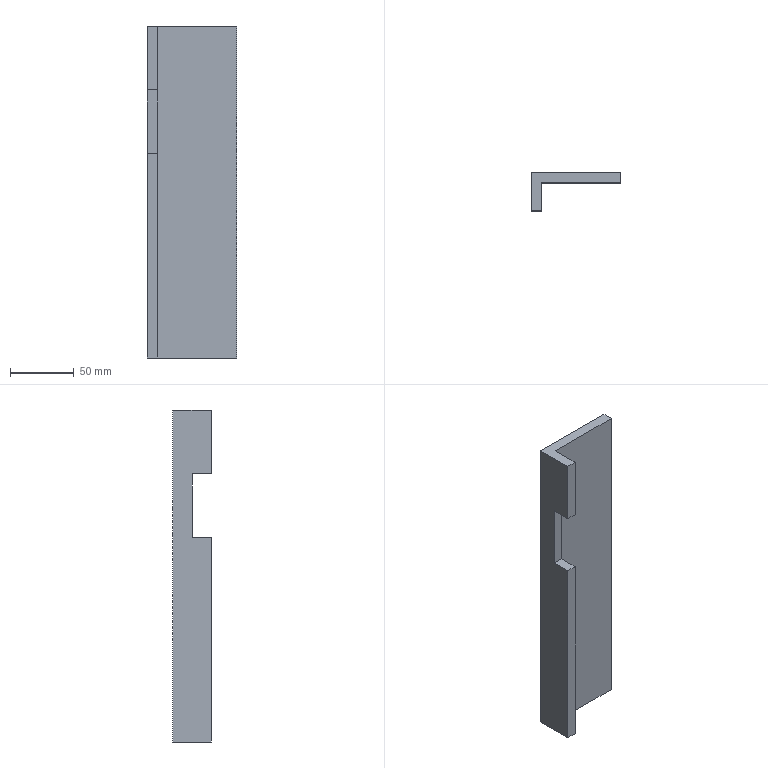Part | SolidWorks | features Cut 1, Extrusion 1 | 1 solid | 12 faces | box 70 x 30 x 260 mm | volume 185360 mm3 | plane 12
STEP:
#1=CARTESIAN_POINT('',(0.,-30.,260.));
#2=VERTEX_POINT('',#1);
#3=CARTESIAN_POINT('',(0.,-30.,210.));
#4=VERTEX_POINT('',#3);
#5=CARTESIAN_POINT('',(0.,-30.,260.));
#6=DIRECTION('',(0.,0.,-1.));
#7=VECTOR('',#6,1000.);
#8=LINE('',#5,#7);
#9=EDGE_CURVE('',#2,#4,#8,.T.);
#10=ORIENTED_EDGE('',*,*,#9,.T.);
#11=CARTESIAN_POINT('',(8.,-30.,210.));
#12=VERTEX_POINT('',#11);
#13=CARTESIAN_POINT('',(10.,-30.,210.));
#14=DIRECTION('',(-1.,0.,0.));
#15=VECTOR('',#14,1000.);
#16=LINE('',#13,#15);
#17=EDGE_CURVE('',#12,#4,#16,.T.);
#18=ORIENTED_EDGE('',*,*,#17,.F.);
#19=CARTESIAN_POINT('',(8.,-30.,260.));
#20=VERTEX_POINT('',#19);
#21=CARTESIAN_POINT('',(8.,-30.,260.));
#22=DIRECTION('',(0.,0.,-1.));
#23=VECTOR('',#22,1000.);
#24=LINE('',#21,#23);
#25=EDGE_CURVE('',#20,#12,#24,.T.);
#26=ORIENTED_EDGE('',*,*,#25,.F.);
#27=CARTESIAN_POINT('',(0.,-30.,260.));
#28=DIRECTION('',(1.,0.,0.));
#29=VECTOR('',#28,1000.);
#30=LINE('',#27,#29);
#31=EDGE_CURVE('',#2,#20,#30,.T.);
#32=ORIENTED_EDGE('',*,*,#31,.F.);
#33=EDGE_LOOP('',(#10,#18,#26,#32));
#34=FACE_OUTER_BOUND('',#33,.T.);
#35=CARTESIAN_POINT('',(0.,-30.,260.));
#36=DIRECTION('',(0.,1.,0.));
#37=DIRECTION('',(0.,0.,1.));
#38=AXIS2_PLACEMENT_3D('',#35,#36,#37);
#39=PLANE('',#38);
#40=ADVANCED_FACE('',(#34),#39,.F.);
#41=CARTESIAN_POINT('',(0.,-15.,210.));
#42=VERTEX_POINT('',#41);
#43=CARTESIAN_POINT('',(0.,-15.,160.));
#44=VERTEX_POINT('',#43);
#45=CARTESIAN_POINT('',(0.,-15.,0.));
#46=DIRECTION('',(0.,0.,-1.));
#47=VECTOR('',#46,1000.);
#48=LINE('',#45,#47);
#49=EDGE_CURVE('',#42,#44,#48,.T.);
#50=ORIENTED_EDGE('',*,*,#49,.F.);
#51=CARTESIAN_POINT('',(0.,0.,210.));
#52=DIRECTION('',(0.,1.,0.));
#53=VECTOR('',#52,1000.);
#54=LINE('',#51,#53);
#55=EDGE_CURVE('',#4,#42,#54,.T.);
#56=ORIENTED_EDGE('',*,*,#55,.F.);
#57=ORIENTED_EDGE('',*,*,#9,.F.);
#58=CARTESIAN_POINT('',(0.,0.,260.));
#59=VERTEX_POINT('',#58);
#60=CARTESIAN_POINT('',(0.,0.,260.));
#61=DIRECTION('',(0.,-1.,0.));
#62=VECTOR('',#61,1000.);
#63=LINE('',#60,#62);
#64=EDGE_CURVE('',#59,#2,#63,.T.);
#65=ORIENTED_EDGE('',*,*,#64,.F.);
#66=CARTESIAN_POINT('',(0.,0.,0.));
#67=VERTEX_POINT('',#66);
#68=CARTESIAN_POINT('',(0.,0.,260.));
#69=DIRECTION('',(0.,0.,-1.));
#70=VECTOR('',#69,1000.);
#71=LINE('',#68,#70);
#72=EDGE_CURVE('',#59,#67,#71,.T.);
#73=ORIENTED_EDGE('',*,*,#72,.T.);
#74=CARTESIAN_POINT('',(0.,-30.,0.));
#75=VERTEX_POINT('',#74);
#76=CARTESIAN_POINT('',(0.,0.,0.));
#77=DIRECTION('',(0.,-1.,0.));
#78=VECTOR('',#77,1000.);
#79=LINE('',#76,#78);
#80=EDGE_CURVE('',#67,#75,#79,.T.);
#81=ORIENTED_EDGE('',*,*,#80,.T.);
#82=CARTESIAN_POINT('',(0.,-30.,160.));
#83=VERTEX_POINT('',#82);
#84=CARTESIAN_POINT('',(0.,-30.,260.));
#85=DIRECTION('',(0.,0.,-1.));
#86=VECTOR('',#85,1000.);
#87=LINE('',#84,#86);
#88=EDGE_CURVE('',#83,#75,#87,.T.);
#89=ORIENTED_EDGE('',*,*,#88,.F.);
#90=CARTESIAN_POINT('',(0.,0.,160.));
#91=DIRECTION('',(0.,-1.,0.));
#92=VECTOR('',#91,1000.);
#93=LINE('',#90,#92);
#94=EDGE_CURVE('',#44,#83,#93,.T.);
#95=ORIENTED_EDGE('',*,*,#94,.F.);
#96=EDGE_LOOP('',(#50,#56,#57,#65,#73,#81,#89,#95));
#97=FACE_OUTER_BOUND('',#96,.T.);
#98=CARTESIAN_POINT('',(0.,0.,260.));
#99=DIRECTION('',(1.,0.,0.));
#100=DIRECTION('',(0.,1.,0.));
#101=AXIS2_PLACEMENT_3D('',#98,#99,#100);
#102=PLANE('',#101);
#103=ADVANCED_FACE('',(#97),#102,.F.);
#104=CARTESIAN_POINT('',(8.,-30.,160.));
#105=VERTEX_POINT('',#104);
#106=CARTESIAN_POINT('',(8.,-30.,0.));
#107=VERTEX_POINT('',#106);
#108=CARTESIAN_POINT('',(8.,-30.,260.));
#109=DIRECTION('',(0.,0.,-1.));
#110=VECTOR('',#109,1000.);
#111=LINE('',#108,#110);
#112=EDGE_CURVE('',#105,#107,#111,.T.);
#113=ORIENTED_EDGE('',*,*,#112,.F.);
#114=CARTESIAN_POINT('',(10.,-30.,160.));
#115=DIRECTION('',(-1.,0.,0.));
#116=VECTOR('',#115,1000.);
#117=LINE('',#114,#116);
#118=EDGE_CURVE('',#105,#83,#117,.T.);
#119=ORIENTED_EDGE('',*,*,#118,.T.);
#120=ORIENTED_EDGE('',*,*,#88,.T.);
#121=CARTESIAN_POINT('',(0.,-30.,0.));
#122=DIRECTION('',(1.,0.,0.));
#123=VECTOR('',#122,1000.);
#124=LINE('',#121,#123);
#125=EDGE_CURVE('',#75,#107,#124,.T.);
#126=ORIENTED_EDGE('',*,*,#125,.T.);
#127=EDGE_LOOP('',(#113,#119,#120,#126));
#128=FACE_OUTER_BOUND('',#127,.T.);
#129=CARTESIAN_POINT('',(0.,-30.,260.));
#130=DIRECTION('',(0.,1.,0.));
#131=DIRECTION('',(0.,0.,1.));
#132=AXIS2_PLACEMENT_3D('',#129,#130,#131);
#133=PLANE('',#132);
#134=ADVANCED_FACE('',(#128),#133,.F.);
#135=ORIENTED_EDGE('',*,*,#25,.T.);
#136=CARTESIAN_POINT('',(8.,-15.,210.));
#137=VERTEX_POINT('',#136);
#138=CARTESIAN_POINT('',(8.,-8.,210.));
#139=DIRECTION('',(0.,1.,0.));
#140=VECTOR('',#139,1000.);
#141=LINE('',#138,#140);
#142=EDGE_CURVE('',#12,#137,#141,.T.);
#143=ORIENTED_EDGE('',*,*,#142,.T.);
#144=CARTESIAN_POINT('',(8.,-15.,160.));
#145=VERTEX_POINT('',#144);
#146=CARTESIAN_POINT('',(8.,-15.,260.));
#147=DIRECTION('',(0.,0.,-1.));
#148=VECTOR('',#147,1000.);
#149=LINE('',#146,#148);
#150=EDGE_CURVE('',#137,#145,#149,.T.);
#151=ORIENTED_EDGE('',*,*,#150,.T.);
#152=CARTESIAN_POINT('',(8.,-8.,160.));
#153=DIRECTION('',(0.,-1.,0.));
#154=VECTOR('',#153,1000.);
#155=LINE('',#152,#154);
#156=EDGE_CURVE('',#145,#105,#155,.T.);
#157=ORIENTED_EDGE('',*,*,#156,.T.);
#158=ORIENTED_EDGE('',*,*,#112,.T.);
#159=CARTESIAN_POINT('',(8.,-8.,0.));
#160=VERTEX_POINT('',#159);
#161=CARTESIAN_POINT('',(8.,-8.,0.));
#162=DIRECTION('',(0.,1.,0.));
#163=VECTOR('',#162,1000.);
#164=LINE('',#161,#163);
#165=EDGE_CURVE('',#107,#160,#164,.T.);
#166=ORIENTED_EDGE('',*,*,#165,.T.);
#167=CARTESIAN_POINT('',(8.,-8.,260.));
#168=VERTEX_POINT('',#167);
#169=CARTESIAN_POINT('',(8.,-8.,260.));
#170=DIRECTION('',(0.,0.,-1.));
#171=VECTOR('',#170,1000.);
#172=LINE('',#169,#171);
#173=EDGE_CURVE('',#168,#160,#172,.T.);
#174=ORIENTED_EDGE('',*,*,#173,.F.);
#175=CARTESIAN_POINT('',(8.,-8.,260.));
#176=DIRECTION('',(0.,1.,0.));
#177=VECTOR('',#176,1000.);
#178=LINE('',#175,#177);
#179=EDGE_CURVE('',#20,#168,#178,.T.);
#180=ORIENTED_EDGE('',*,*,#179,.F.);
#181=EDGE_LOOP('',(#135,#143,#151,#157,#158,#166,#174,#180));
#182=FACE_OUTER_BOUND('',#181,.T.);
#183=CARTESIAN_POINT('',(8.,-8.,260.));
#184=DIRECTION('',(-1.,0.,0.));
#185=DIRECTION('',(0.,0.,1.));
#186=AXIS2_PLACEMENT_3D('',#183,#184,#185);
#187=PLANE('',#186);
#188=ADVANCED_FACE('',(#182),#187,.F.);
#189=CARTESIAN_POINT('',(70.,-8.,0.));
#190=VERTEX_POINT('',#189);
#191=CARTESIAN_POINT('',(8.,-8.,0.));
#192=DIRECTION('',(1.,0.,0.));
#193=VECTOR('',#192,1000.);
#194=LINE('',#191,#193);
#195=EDGE_CURVE('',#160,#190,#194,.T.);
#196=ORIENTED_EDGE('',*,*,#195,.T.);
#197=CARTESIAN_POINT('',(70.,-8.,260.));
#198=VERTEX_POINT('',#197);
#199=CARTESIAN_POINT('',(70.,-8.,260.));
#200=DIRECTION('',(0.,0.,-1.));
#201=VECTOR('',#200,1000.);
#202=LINE('',#199,#201);
#203=EDGE_CURVE('',#198,#190,#202,.T.);
#204=ORIENTED_EDGE('',*,*,#203,.F.);
#205=CARTESIAN_POINT('',(8.,-8.,260.));
#206=DIRECTION('',(1.,0.,0.));
#207=VECTOR('',#206,1000.);
#208=LINE('',#205,#207);
#209=EDGE_CURVE('',#168,#198,#208,.T.);
#210=ORIENTED_EDGE('',*,*,#209,.F.);
#211=ORIENTED_EDGE('',*,*,#173,.T.);
#212=EDGE_LOOP('',(#196,#204,#210,#211));
#213=FACE_OUTER_BOUND('',#212,.T.);
#214=CARTESIAN_POINT('',(8.,-8.,260.));
#215=DIRECTION('',(0.,1.,0.));
#216=DIRECTION('',(0.,0.,1.));
#217=AXIS2_PLACEMENT_3D('',#214,#215,#216);
#218=PLANE('',#217);
#219=ADVANCED_FACE('',(#213),#218,.F.);
#220=CARTESIAN_POINT('',(70.,0.,0.));
#221=VERTEX_POINT('',#220);
#222=CARTESIAN_POINT('',(70.,-8.,0.));
#223=DIRECTION('',(0.,1.,0.));
#224=VECTOR('',#223,1000.);
#225=LINE('',#222,#224);
#226=EDGE_CURVE('',#190,#221,#225,.T.);
#227=ORIENTED_EDGE('',*,*,#226,.T.);
#228=CARTESIAN_POINT('',(70.,0.,260.));
#229=VERTEX_POINT('',#228);
#230=CARTESIAN_POINT('',(70.,0.,260.));
#231=DIRECTION('',(0.,0.,-1.));
#232=VECTOR('',#231,1000.);
#233=LINE('',#230,#232);
#234=EDGE_CURVE('',#229,#221,#233,.T.);
#235=ORIENTED_EDGE('',*,*,#234,.F.);
#236=CARTESIAN_POINT('',(70.,-8.,260.));
#237=DIRECTION('',(0.,1.,0.));
#238=VECTOR('',#237,1000.);
#239=LINE('',#236,#238);
#240=EDGE_CURVE('',#198,#229,#239,.T.);
#241=ORIENTED_EDGE('',*,*,#240,.F.);
#242=ORIENTED_EDGE('',*,*,#203,.T.);
#243=EDGE_LOOP('',(#227,#235,#241,#242));
#244=FACE_OUTER_BOUND('',#243,.T.);
#245=CARTESIAN_POINT('',(70.,-8.,260.));
#246=DIRECTION('',(-1.,0.,0.));
#247=DIRECTION('',(0.,0.,1.));
#248=AXIS2_PLACEMENT_3D('',#245,#246,#247);
#249=PLANE('',#248);
#250=ADVANCED_FACE('',(#244),#249,.F.);
#251=CARTESIAN_POINT('',(0.,0.,0.));
#252=DIRECTION('',(-1.,0.,0.));
#253=VECTOR('',#252,1000.);
#254=LINE('',#251,#253);
#255=EDGE_CURVE('',#221,#67,#254,.T.);
#256=ORIENTED_EDGE('',*,*,#255,.T.);
#257=ORIENTED_EDGE('',*,*,#72,.F.);
#258=CARTESIAN_POINT('',(0.,0.,260.));
#259=DIRECTION('',(-1.,0.,0.));
#260=VECTOR('',#259,1000.);
#261=LINE('',#258,#260);
#262=EDGE_CURVE('',#229,#59,#261,.T.);
#263=ORIENTED_EDGE('',*,*,#262,.F.);
#264=ORIENTED_EDGE('',*,*,#234,.T.);
#265=EDGE_LOOP('',(#256,#257,#263,#264));
#266=FACE_OUTER_BOUND('',#265,.T.);
#267=CARTESIAN_POINT('',(0.,0.,260.));
#268=DIRECTION('',(0.,-1.,0.));
#269=DIRECTION('',(0.,0.,-1.));
#270=AXIS2_PLACEMENT_3D('',#267,#268,#269);
#271=PLANE('',#270);
#272=ADVANCED_FACE('',(#266),#271,.F.);
#273=ORIENTED_EDGE('',*,*,#64,.T.);
#274=ORIENTED_EDGE('',*,*,#31,.T.);
#275=ORIENTED_EDGE('',*,*,#179,.T.);
#276=ORIENTED_EDGE('',*,*,#209,.T.);
#277=ORIENTED_EDGE('',*,*,#240,.T.);
#278=ORIENTED_EDGE('',*,*,#262,.T.);
#279=EDGE_LOOP('',(#273,#274,#275,#276,#277,#278));
#280=FACE_OUTER_BOUND('',#279,.T.);
#281=CARTESIAN_POINT('',(0.,0.,260.));
#282=DIRECTION('',(0.,0.,1.));
#283=DIRECTION('',(1.,0.,0.));
#284=AXIS2_PLACEMENT_3D('',#281,#282,#283);
#285=PLANE('',#284);
#286=ADVANCED_FACE('',(#280),#285,.T.);
#287=ORIENTED_EDGE('',*,*,#80,.F.);
#288=ORIENTED_EDGE('',*,*,#255,.F.);
#289=ORIENTED_EDGE('',*,*,#226,.F.);
#290=ORIENTED_EDGE('',*,*,#195,.F.);
#291=ORIENTED_EDGE('',*,*,#165,.F.);
#292=ORIENTED_EDGE('',*,*,#125,.F.);
#293=EDGE_LOOP('',(#287,#288,#289,#290,#291,#292));
#294=FACE_OUTER_BOUND('',#293,.T.);
#295=CARTESIAN_POINT('',(0.,0.,0.));
#296=DIRECTION('',(0.,0.,1.));
#297=DIRECTION('',(1.,0.,0.));
#298=AXIS2_PLACEMENT_3D('',#295,#296,#297);
#299=PLANE('',#298);
#300=ADVANCED_FACE('',(#294),#299,.F.);
#301=CARTESIAN_POINT('',(10.,-15.,210.));
#302=DIRECTION('',(-1.,0.,0.));
#303=VECTOR('',#302,1000.);
#304=LINE('',#301,#303);
#305=EDGE_CURVE('',#137,#42,#304,.T.);
#306=ORIENTED_EDGE('',*,*,#305,.T.);
#307=ORIENTED_EDGE('',*,*,#49,.T.);
#308=CARTESIAN_POINT('',(10.,-15.,160.));
#309=DIRECTION('',(-1.,0.,0.));
#310=VECTOR('',#309,1000.);
#311=LINE('',#308,#310);
#312=EDGE_CURVE('',#145,#44,#311,.T.);
#313=ORIENTED_EDGE('',*,*,#312,.F.);
#314=ORIENTED_EDGE('',*,*,#150,.F.);
#315=EDGE_LOOP('',(#306,#307,#313,#314));
#316=FACE_OUTER_BOUND('',#315,.T.);
#317=CARTESIAN_POINT('',(10.,-15.,0.));
#318=DIRECTION('',(0.,1.,0.));
#319=DIRECTION('',(0.,0.,1.));
#320=AXIS2_PLACEMENT_3D('',#317,#318,#319);
#321=PLANE('',#320);
#322=ADVANCED_FACE('',(#316),#321,.F.);
#323=ORIENTED_EDGE('',*,*,#17,.T.);
#324=ORIENTED_EDGE('',*,*,#55,.T.);
#325=ORIENTED_EDGE('',*,*,#305,.F.);
#326=ORIENTED_EDGE('',*,*,#142,.F.);
#327=EDGE_LOOP('',(#323,#324,#325,#326));
#328=FACE_OUTER_BOUND('',#327,.T.);
#329=CARTESIAN_POINT('',(10.,0.,210.));
#330=DIRECTION('',(0.,0.,1.));
#331=DIRECTION('',(1.,0.,0.));
#332=AXIS2_PLACEMENT_3D('',#329,#330,#331);
#333=PLANE('',#332);
#334=ADVANCED_FACE('',(#328),#333,.F.);
#335=ORIENTED_EDGE('',*,*,#312,.T.);
#336=ORIENTED_EDGE('',*,*,#94,.T.);
#337=ORIENTED_EDGE('',*,*,#118,.F.);
#338=ORIENTED_EDGE('',*,*,#156,.F.);
#339=EDGE_LOOP('',(#335,#336,#337,#338));
#340=FACE_OUTER_BOUND('',#339,.T.);
#341=CARTESIAN_POINT('',(10.,0.,160.));
#342=DIRECTION('',(0.,0.,-1.));
#343=DIRECTION('',(-1.,0.,0.));
#344=AXIS2_PLACEMENT_3D('',#341,#342,#343);
#345=PLANE('',#344);
#346=ADVANCED_FACE('',(#340),#345,.F.);
#347=CLOSED_SHELL('',(#40,#103,#134,#188,#219,#250,#272,#286,#300,#322,#334,#346));
#348=MANIFOLD_SOLID_BREP('',#347);
#349=CARTESIAN_POINT('',(0.,0.,0.));
#350=DIRECTION('',(0.,0.,1.));
#351=DIRECTION('',(1.,0.,0.));
#352=AXIS2_PLACEMENT_3D('',#349,#350,#351);
#353=(LENGTH_UNIT()NAMED_UNIT(*)SI_UNIT(.MILLI.,.METRE.));
#354=UNCERTAINTY_MEASURE_WITH_UNIT(LENGTH_MEASURE(0.00001),#353,'','');
#355=(NAMED_UNIT(*)PLANE_ANGLE_UNIT()SI_UNIT($,.RADIAN.));
#356=(NAMED_UNIT(*)SI_UNIT($,.STERADIAN.)SOLID_ANGLE_UNIT());
#357=(GEOMETRIC_REPRESENTATION_CONTEXT(3)GLOBAL_UNCERTAINTY_ASSIGNED_CONTEXT((#354))GLOBAL_UNIT_ASSIGNED_CONTEXT((#353,#355,#356))REPRESENTATION_CONTEXT('',''));
#358=ADVANCED_BREP_SHAPE_REPRESENTATION('',(#348,#352),#357);